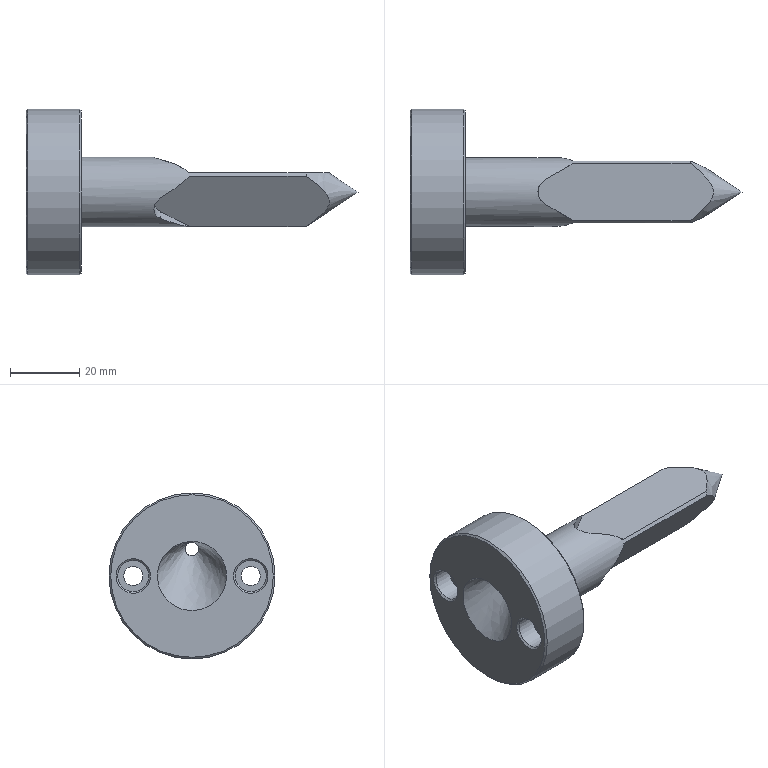NC program | NX | posted with a generic post | part box 96 x 48 x 48 mm
Lines 1 to 853 of 9730:
N10 G17 G21 G94 G90
(ZLEVEL_PROFILE , TOOL : D8)
N12 T08 M6
N14 G54
N16 G17 G0 G90 X5.071 Y-2.683 B0. C0. S3500 M3
N18 G43 Z30. H8
N20 Z1.5
N22 G94 G1 X5.428 Y-2.048 Z1.462 F1000.
N24 X5.805 Y-0.502 Z1.378
N26 X5.75 Y1.087 Z1.295
N28 X5.431 Y2.226 Z1.233
N30 X4.665 Y3.598 Z1.151
N32 X3.56 Y4.716 Z1.068
N34 X2.196 Y5.499 Z0.986
N36 X0.673 Y5.889 Z0.904
N38 X-0.898 Y5.858 Z0.821
N40 X-2.405 Y5.41 Z0.739
N42 X-3.737 Y4.575 Z0.656
N44 X-4.563 Y3.73 Z0.595
N46 X-5.369 Y2.38 Z0.512
N48 X-5.785 Y0.864 Z0.43
N50 X-5.781 Y-0.708 Z0.347
N52 X-5.357 Y-2.222 Z0.265
N54 X-4.545 Y-3.568 Z0.183
N56 X-3.403 Y-4.648 Z0.1
N58 X-2.014 Y-5.384 Z0.018
N60 X-0.869 Y-5.678 Z-0.044
N62 X-0.591 Y-5.713 Z-0.059
N64 X0. Z-0.09
N66 G3 X5.805 Y0.093 R5.805 F2200.
N68 X0. Y-5.713 R-5.805
N70 G1 X0.32 Y-5.694 Z-0.095
N72 X0.639 Y-5.66 Z-0.101
N74 X0.955 Y-5.609 Z-0.107
N76 X1.267 Y-5.538 Z-0.112
N78 X1.575 Y-5.454 Z-0.118
N80 X1.877 Y-5.349 Z-0.123
N82 X2.173 Y-5.232 Z-0.129
N84 X2.46 Y-5.093 Z-0.135
N86 X2.742 Y-4.948 Z-0.14
N88 X3.01 Y-4.777 Z-0.146
N90 X3.276 Y-4.605 Z-0.151
N92 X3.523 Y-4.406 Z-0.157
N94 X3.769 Y-4.207 Z-0.163
N96 X3.991 Y-3.982 Z-0.168
N98 X4.214 Y-3.758 Z-0.174
N100 X4.419 Y-3.517 Z-0.18
N102 G3 X0. Y-5.593 R-5.742
N104 G1 X0.32 Y-5.575 Z-0.185
N106 X0.639 Y-5.54 Z-0.191
N108 X0.955 Y-5.488 Z-0.196
N110 X1.267 Y-5.416 Z-0.202
N112 X1.575 Y-5.332 Z-0.208
N114 X1.876 Y-5.225 Z-0.213
N116 X2.171 Y-5.107 Z-0.219
N118 X2.458 Y-4.967 Z-0.224
N120 X2.739 Y-4.821 Z-0.23
N122 X3.006 Y-4.648 Z-0.236
N124 X3.271 Y-4.475 Z-0.241
N126 X3.516 Y-4.273 Z-0.247
N128 X3.761 Y-4.073 Z-0.252
N130 X3.981 Y-3.845 Z-0.258
N132 X4.203 Y-3.62 Z-0.264
N134 X4.406 Y-3.378 Z-0.269
N136 G3 X0. Y-5.473 R-5.681
N138 G1 X0.32 Y-5.455 Z-0.275
N140 X0.639 Y-5.42 Z-0.281
N142 X0.955 Y-5.366 Z-0.286
N144 X1.267 Y-5.294 Z-0.292
N146 X1.574 Y-5.21 Z-0.297
N148 X1.875 Y-5.101 Z-0.303
N150 X2.169 Y-4.981 Z-0.309
N152 X2.456 Y-4.842 Z-0.314
N154 X2.736 Y-4.692 Z-0.32
N156 X3.002 Y-4.519 Z-0.325
N158 X3.265 Y-4.343 Z-0.331
N160 X3.509 Y-4.14 Z-0.337
N162 X3.752 Y-3.938 Z-0.342
N164 X3.97 Y-3.709 Z-0.348
N166 X4.191 Y-3.483 Z-0.353
N168 X4.39 Y-3.238 Z-0.359
N170 G3 X0. Y-5.352 R-5.619
N172 G1 X0.32 Y-5.334 Z-0.365
N174 X0.639 Y-5.299 Z-0.37
N176 X0.955 Y-5.245 Z-0.376
N178 X1.267 Y-5.172 Z-0.382
N180 X1.574 Y-5.087 Z-0.387
N182 X1.874 Y-4.977 Z-0.393
N184 X2.168 Y-4.855 Z-0.398
N186 X2.454 Y-4.716 Z-0.404
N188 X2.732 Y-4.563 Z-0.41
N190 X2.999 Y-4.389 Z-0.415
N192 X3.26 Y-4.211 Z-0.421
N194 X3.503 Y-4.007 Z-0.426
N196 X3.743 Y-3.802 Z-0.432
N198 X3.96 Y-3.571 Z-0.438
N200 X4.179 Y-3.343 Z-0.443
N202 X4.376 Y-3.097 Z-0.449
N204 G3 X0. Y-5.23 R-5.556
N206 G1 X0.32 Y-5.214 Z-0.454
N208 X0.64 Y-5.179 Z-0.46
N210 X0.955 Y-5.123 Z-0.466
N212 X1.267 Y-5.05 Z-0.471
N214 X1.574 Y-4.963 Z-0.477
N216 X1.874 Y-4.853 Z-0.483
N218 X2.167 Y-4.729 Z-0.488
N220 X2.453 Y-4.591 Z-0.494
N222 X2.729 Y-4.434 Z-0.499
N224 X2.996 Y-4.26 Z-0.505
N226 X3.255 Y-4.078 Z-0.511
N228 X3.497 Y-3.874 Z-0.516
N230 X3.734 Y-3.665 Z-0.522
N232 X3.95 Y-3.433 Z-0.527
N234 X4.166 Y-3.203 Z-0.533
N236 X4.36 Y-2.954 Z-0.539
N238 G3 X0. Y-5.11 R-5.493
N240 G1 X0.32 Y-5.094 Z-0.544
N242 X0.639 Y-5.058 Z-0.55
N244 X0.954 Y-5.001 Z-0.555
N246 X1.266 Y-4.927 Z-0.561
N248 X1.573 Y-4.84 Z-0.567
N250 X1.872 Y-4.728 Z-0.572
N252 X2.165 Y-4.603 Z-0.578
N254 X2.451 Y-4.464 Z-0.584
N256 X2.726 Y-4.305 Z-0.589
N258 X2.992 Y-4.132 Z-0.595
N260 X3.248 Y-3.946 Z-0.6
N262 X3.49 Y-3.74 Z-0.606
N264 X3.725 Y-3.529 Z-0.612
N266 X3.938 Y-3.295 Z-0.617
N268 X4.152 Y-3.063 Z-0.623
N270 X4.344 Y-2.812 Z-0.628
N272 G3 X-0.001 Y-4.989 R-5.43
N274 G1 X0.32 Y-4.974 Z-0.634
N276 X0.64 Y-4.938 Z-0.64
N278 X0.954 Y-4.88 Z-0.645
N280 X1.266 Y-4.805 Z-0.651
N282 X1.572 Y-4.716 Z-0.657
N284 X1.871 Y-4.603 Z-0.662
N286 X2.164 Y-4.478 Z-0.668
N288 X2.449 Y-4.336 Z-0.673
N290 X2.723 Y-4.176 Z-0.679
N292 X2.989 Y-4.002 Z-0.685
N294 X3.243 Y-3.813 Z-0.69
N296 X3.483 Y-3.605 Z-0.696
N298 X3.716 Y-3.392 Z-0.701
N300 X3.928 Y-3.157 Z-0.707
N302 X4.139 Y-2.922 Z-0.713
N304 X4.328 Y-2.669 Z-0.718
N306 G3 X-0.001 Y-4.868 R-5.368
N308 G1 X0.32 Y-4.854 Z-0.724
N310 X0.64 Y-4.817 Z-0.729
N312 X0.954 Y-4.758 Z-0.735
N314 X1.266 Y-4.683 Z-0.741
N316 X1.572 Y-4.593 Z-0.746
N318 X1.87 Y-4.477 Z-0.752
N320 X2.163 Y-4.353 Z-0.758
N322 X2.446 Y-4.208 Z-0.763
N324 X2.721 Y-4.048 Z-0.769
N326 X2.985 Y-3.872 Z-0.774
N328 X3.238 Y-3.681 Z-0.78
N330 X3.476 Y-3.472 Z-0.786
N332 X3.707 Y-3.256 Z-0.791
N334 X3.917 Y-3.019 Z-0.797
N336 X4.126 Y-2.781 Z-0.802
N338 X4.315 Y-2.529 Z-0.808
N340 G3 X-0.001 Y-4.749 R-5.306
N342 G1 X0.32 Y-4.734 Z-0.814
N344 X0.639 Y-4.697 Z-0.819
N346 X0.954 Y-4.637 Z-0.825
N348 X1.265 Y-4.562 Z-0.831
N350 X1.571 Y-4.47 Z-0.836
N352 X1.868 Y-4.352 Z-0.842
N354 X2.16 Y-4.227 Z-0.847
N356 X2.442 Y-4.08 Z-0.853
N358 X2.716 Y-3.919 Z-0.859
N360 X2.979 Y-3.741 Z-0.864
N362 X3.23 Y-3.549 Z-0.87
N364 X3.468 Y-3.339 Z-0.875
N366 X3.696 Y-3.121 Z-0.881
N368 X3.904 Y-2.883 Z-0.887
N370 X4.109 Y-2.643 Z-0.892
N372 X4.297 Y-2.389 Z-0.898
N374 G3 X-0.001 Y-4.632 R-5.246
N376 G1 X0.32 Y-4.614 Z-0.904
N378 X0.639 Y-4.576 Z-0.909
N380 X0.953 Y-4.515 Z-0.915
N382 X1.264 Y-4.44 Z-0.92
N384 X1.569 Y-4.347 Z-0.926
N386 X1.865 Y-4.228 Z-0.932
N388 X2.157 Y-4.102 Z-0.937
N390 X2.438 Y-3.952 Z-0.943
N392 X2.711 Y-3.791 Z-0.948
N394 X2.972 Y-3.61 Z-0.954
N396 X3.223 Y-3.417 Z-0.96
N398 X3.46 Y-3.207 Z-0.965
N400 X3.685 Y-2.986 Z-0.971
N402 X3.891 Y-2.746 Z-0.976
N404 X4.093 Y-2.503 Z-0.982
N406 X4.277 Y-2.247 Z-0.988
N408 G3 X-0.001 Y-4.507 R-5.182
N410 G1 X0.32 Y-4.494 Z-0.993
N412 X0.639 Y-4.455 Z-0.999
N414 X0.954 Y-4.394 Z-1.005
N416 X1.265 Y-4.318 Z-1.01
N418 X1.569 Y-4.223 Z-1.016
N420 X1.865 Y-4.101 Z-1.021
N422 X2.157 Y-3.975 Z-1.027
N424 X2.436 Y-3.822 Z-1.033
N426 X2.709 Y-3.661 Z-1.038
N428 X2.968 Y-3.477 Z-1.044
N430 X3.218 Y-3.283 Z-1.049
N432 X3.453 Y-3.07 Z-1.055
N434 X3.676 Y-2.847 Z-1.061
N436 X3.882 Y-2.607 Z-1.066
N438 X4.078 Y-2.359 Z-1.072
N440 X4.259 Y-2.1 Z-1.078
N442 G3 X-0.001 Y-4.384 R-5.118
N444 G1 X0.32 Y-4.374 Z-1.083
N446 X0.64 Y-4.335 Z-1.089
N448 X0.954 Y-4.272 Z-1.094
N450 X1.265 Y-4.196 Z-1.1
N452 X1.569 Y-4.099 Z-1.106
N454 X1.864 Y-3.975 Z-1.111
N456 X2.156 Y-3.849 Z-1.117
N458 X2.434 Y-3.693 Z-1.122
N460 X2.707 Y-3.531 Z-1.128
N462 X2.964 Y-3.344 Z-1.134
N464 X3.213 Y-3.15 Z-1.139
N466 X3.445 Y-2.933 Z-1.145
N468 X3.666 Y-2.708 Z-1.151
N470 X3.871 Y-2.466 Z-1.156
N472 X4.063 Y-2.216 Z-1.162
N474 X4.24 Y-1.955 Z-1.167
N476 G3 X-0.001 Y-4.266 R-5.058
N478 G1 X0.32 Y-4.253 Z-1.173
N480 X0.639 Y-4.214 Z-1.179
N482 X0.953 Y-4.15 Z-1.184
N484 X1.265 Y-4.074 Z-1.19
N486 X1.567 Y-3.974 Z-1.195
N488 X1.862 Y-3.849 Z-1.201
N490 X2.154 Y-3.723 Z-1.207
N492 X2.43 Y-3.564 Z-1.212
N494 X2.703 Y-3.403 Z-1.218
N496 X2.957 Y-3.213 Z-1.224
N498 X3.206 Y-3.017 Z-1.229
N500 X3.434 Y-2.797 Z-1.235
N502 X3.655 Y-2.571 Z-1.24
N504 X3.855 Y-2.326 Z-1.246
N506 X4.047 Y-2.076 Z-1.252
N508 X4.219 Y-1.811 Z-1.257
N510 G3 X-0.001 Y-4.144 R-4.995
N512 G1 X0.32 Y-4.133 Z-1.263
N514 X0.639 Y-4.093 Z-1.268
N516 X0.953 Y-4.028 Z-1.274
N518 X1.265 Y-3.953 Z-1.28
N520 X1.566 Y-3.848 Z-1.285
N522 X1.861 Y-3.723 Z-1.291
N524 X2.152 Y-3.596 Z-1.297
N526 X2.427 Y-3.436 Z-1.302
N528 X2.699 Y-3.272 Z-1.308
N530 X2.951 Y-3.079 Z-1.313
N532 X3.199 Y-2.882 Z-1.319
N534 X3.424 Y-2.659 Z-1.325
N536 X3.646 Y-2.433 Z-1.33
N538 X3.839 Y-2.183 Z-1.336
N540 X4.032 Y-1.933 Z-1.341
N542 X4.203 Y-1.667 Z-1.347
N544 G3 X-0.001 Y-4.025 R-4.933
N546 G1 X0.32 Y-4.013 Z-1.353
N548 X0.639 Y-3.973 Z-1.358
N550 X0.952 Y-3.906 Z-1.364
N552 X1.264 Y-3.831 Z-1.37
N554 X1.564 Y-3.723 Z-1.375
N556 X1.859 Y-3.599 Z-1.381
N558 X2.148 Y-3.468 Z-1.386
N560 X2.423 Y-3.308 Z-1.392
N562 X2.693 Y-3.141 Z-1.398
N564 X2.943 Y-2.946 Z-1.403
N566 X3.189 Y-2.747 Z-1.409
N568 X3.411 Y-2.522 Z-1.414
N570 X3.632 Y-2.296 Z-1.42
N572 X3.821 Y-2.042 Z-1.426
N574 X4.013 Y-1.792 Z-1.431
N576 X4.184 Y-1.527 Z-1.437
N578 G3 X-0.001 Y-3.907 R-4.875
N580 G1 X0.32 Y-3.893 Z-1.443
N582 X0.639 Y-3.852 Z-1.448
N584 X0.952 Y-3.784 Z-1.454
N586 X1.263 Y-3.709 Z-1.459
N588 X1.562 Y-3.598 Z-1.465
N590 X1.857 Y-3.475 Z-1.471
N592 X2.144 Y-3.34 Z-1.476
N594 X2.418 Y-3.18 Z-1.482
N596 X2.686 Y-3.01 Z-1.487
N598 X2.936 Y-2.814 Z-1.493
N600 X3.178 Y-2.612 Z-1.499
N602 X3.398 Y-2.385 Z-1.504
N604 X3.616 Y-2.158 Z-1.51
N606 X3.802 Y-1.902 Z-1.516
N608 X3.992 Y-1.65 Z-1.521
N610 X4.157 Y-1.382 Z-1.527
N612 G3 X4.478 Y2.777 R4.813
N614 X-4.702 Y2.09 R4.818
N616 X-0.001 Y-3.782 R4.813
N618 G1 X0.32 Y-3.773 Z-1.532
N620 X0.639 Y-3.731 Z-1.538
N622 X0.952 Y-3.661 Z-1.544
N624 X1.264 Y-3.586 Z-1.549
N626 X1.562 Y-3.473 Z-1.555
N628 X1.857 Y-3.35 Z-1.561
N630 X2.143 Y-3.21 Z-1.566
N632 X2.417 Y-3.049 Z-1.572
N634 X2.682 Y-2.875 Z-1.577
N636 X2.931 Y-2.679 Z-1.583
N638 X3.171 Y-2.474 Z-1.589
N640 X3.39 Y-2.245 Z-1.594
N642 X3.605 Y-2.014 Z-1.6
N644 X3.788 Y-1.757 Z-1.605
N646 X3.976 Y-1.503 Z-1.611
N648 X4.139 Y-1.233 Z-1.617
N650 G3 X-0.002 Y-3.665 R-4.747
N652 G1 X0.32 Y-3.653 Z-1.622
N654 X0.639 Y-3.61 Z-1.628
N656 X0.951 Y-3.539 Z-1.634
N658 X1.263 Y-3.464 Z-1.639
N660 X1.56 Y-3.348 Z-1.645
N662 X1.854 Y-3.225 Z-1.65
N664 X2.137 Y-3.082 Z-1.656
N666 X2.411 Y-2.921 Z-1.662
N668 X2.674 Y-2.744 Z-1.667
N670 X2.921 Y-2.546 Z-1.673
N672 X3.16 Y-2.34 Z-1.678
N674 X3.376 Y-2.109 Z-1.684
N676 X3.59 Y-1.877 Z-1.69
N678 X3.769 Y-1.618 Z-1.695
N680 X3.956 Y-1.363 Z-1.701
N682 X4.114 Y-1.09 Z-1.707
N684 G3 X-0.002 Y-3.547 R-4.687
N686 G1 X0.319 Y-3.533 Z-1.712
N688 X0.638 Y-3.489 Z-1.718
N690 X0.95 Y-3.418 Z-1.723
N692 X1.261 Y-3.341 Z-1.729
N694 X1.557 Y-3.222 Z-1.735
N696 X1.851 Y-3.099 Z-1.74
N698 X2.133 Y-2.953 Z-1.746
N700 X2.407 Y-2.793 Z-1.751
N702 X2.667 Y-2.613 Z-1.757
N704 X2.913 Y-2.414 Z-1.763
N706 X3.15 Y-2.205 Z-1.768
N708 X3.364 Y-1.972 Z-1.774
N710 X3.576 Y-1.739 Z-1.78
N712 X3.753 Y-1.478 Z-1.785
N714 X3.934 Y-1.219 Z-1.791
N716 X4.085 Y-0.943 Z-1.796
N718 G3 X-0.002 Y-3.421 R-4.622
N720 G1 X0.32 Y-3.412 Z-1.802
N722 X0.639 Y-3.367 Z-1.808
N724 X0.951 Y-3.296 Z-1.813
N726 X1.262 Y-3.217 Z-1.819
N728 X1.557 Y-3.095 Z-1.825
N730 X1.852 Y-2.973 Z-1.83
N732 X2.132 Y-2.824 Z-1.836
N734 X2.405 Y-2.661 Z-1.841
N736 X2.665 Y-2.48 Z-1.847
N738 X2.909 Y-2.278 Z-1.853
N740 X3.145 Y-2.068 Z-1.858
N742 X3.356 Y-1.832 Z-1.864
N744 X3.566 Y-1.596 Z-1.869
N746 X3.742 Y-1.334 Z-1.875
N748 X3.914 Y-1.069 Z-1.881
N750 X4.066 Y-0.792 Z-1.886
N752 G3 X-0.002 Y-3.301 R-4.561
N754 G1 X0.319 Y-3.292 Z-1.892
N756 X0.638 Y-3.246 Z-1.898
N758 X0.951 Y-3.174 Z-1.903
N760 X1.261 Y-3.093 Z-1.909
N762 X1.555 Y-2.97 Z-1.914
N764 X1.85 Y-2.847 Z-1.92
N766 X2.129 Y-2.697 Z-1.926
N768 X2.401 Y-2.532 Z-1.931
N770 X2.66 Y-2.35 Z-1.937
N772 X2.902 Y-2.146 Z-1.943
N774 X3.137 Y-1.935 Z-1.948
N776 X3.346 Y-1.697 Z-1.954
N778 X3.549 Y-1.456 Z-1.959
N780 X3.724 Y-1.193 Z-1.965
N782 X3.891 Y-0.925 Z-1.971
N784 X4.041 Y-0.648 Z-1.976
N786 G3 X-0.002 Y-3.179 R-4.499
N788 G1 X0.32 Y-3.172 Z-1.982
N790 X0.638 Y-3.124 Z-1.987
N792 X0.951 Y-3.053 Z-1.993
N794 X1.26 Y-2.968 Z-1.999
N796 X1.554 Y-2.844 Z-2.004
N798 X1.848 Y-2.721 Z-2.01
N800 X2.127 Y-2.569 Z-2.016
N802 X2.397 Y-2.403 Z-2.021
N804 X2.656 Y-2.22 Z-2.027
N806 X2.896 Y-2.013 Z-2.032
N808 X3.127 Y-1.798 Z-2.038
N810 X3.337 Y-1.561 Z-2.044
N812 X3.533 Y-1.314 Z-2.049
N814 X3.706 Y-1.05 Z-2.055
N816 X3.869 Y-0.78 Z-2.061
N818 X4.011 Y-0.499 Z-2.066
N820 G3 X-0.002 Y-3.058 R-4.434
N822 G1 X0.319 Y-3.052 Z-2.072
N824 X0.638 Y-3.002 Z-2.077
N826 X0.95 Y-2.932 Z-2.083
N828 X1.259 Y-2.843 Z-2.089
N830 X1.553 Y-2.719 Z-2.094
N832 X1.846 Y-2.595 Z-2.1
N834 X2.125 Y-2.442 Z-2.105
N836 X2.394 Y-2.273 Z-2.111
N838 X2.652 Y-2.09 Z-2.117
N840 X2.89 Y-1.88 Z-2.122
N842 X3.117 Y-1.66 Z-2.128
N844 X3.324 Y-1.421 Z-2.134
N846 X3.518 Y-1.172 Z-2.139
N848 X3.682 Y-0.903 Z-2.145
N850 X3.849 Y-0.634 Z-2.15
N852 X3.987 Y-0.351 Z-2.156
N854 G3 X-0.002 Y-2.942 R-4.376
N856 G1 X0.319 Y-2.932 Z-2.162
N858 X0.637 Y-2.881 Z-2.167
N860 X0.949 Y-2.811 Z-2.173
N862 X1.256 Y-2.718 Z-2.179
N864 X1.55 Y-2.596 Z-2.184
N866 X1.843 Y-2.469 Z-2.19
N868 X2.121 Y-2.317 Z-2.195
N870 X2.387 Y-2.144 Z-2.201
N872 X2.643 Y-1.958 Z-2.207
N874 X2.879 Y-1.747 Z-2.212
N876 X3.104 Y-1.525 Z-2.218
N878 X3.305 Y-1.282 Z-2.223
N880 X3.5 Y-1.034 Z-2.229
N882 X3.657 Y-0.76 Z-2.235
N884 X3.823 Y-0.491 Z-2.24
N886 X3.961 Y-0.208 Z-2.246
N888 G3 X-0.002 Y-2.82 R-4.315
N890 G1 X0.319 Y-2.811 Z-2.252
N892 X0.637 Y-2.759 Z-2.257
N894 X0.949 Y-2.69 Z-2.263
N896 X1.255 Y-2.593 Z-2.268
N898 X1.549 Y-2.472 Z-2.274
N900 X1.84 Y-2.341 Z-2.28
N902 X2.119 Y-2.192 Z-2.285
N904 X2.382 Y-2.013 Z-2.291
N906 X2.636 Y-1.825 Z-2.297
N908 X2.871 Y-1.612 Z-2.302
N910 X3.093 Y-1.389 Z-2.308
N912 X3.288 Y-1.14 Z-2.313
N914 X3.483 Y-0.892 Z-2.319
N916 X3.659 Y-0.63 Z-2.325
N918 X3.798 Y-0.348 Z-2.33
N920 X3.925 Y-0.059 Z-2.336
N922 G3 X-0.003 Y-2.695 R-4.25
N924 G1 X0.319 Y-2.691 Z-2.342
N926 X0.638 Y-2.637 Z-2.347
N928 X0.95 Y-2.569 Z-2.353
N930 X1.255 Y-2.466 Z-2.358
N932 X1.55 Y-2.348 Z-2.364
N934 X1.839 Y-2.211 Z-2.37
N936 X2.119 Y-2.063 Z-2.375
N938 X2.379 Y-1.88 Z-2.381
N940 X2.632 Y-1.69 Z-2.386
N942 X2.862 Y-1.472 Z-2.392
N944 X3.084 Y-1.248 Z-2.398
N946 X3.274 Y-0.994 Z-2.403
N948 X3.468 Y-0.746 Z-2.409
N950 X3.616 Y-0.467 Z-2.415
N952 X3.773 Y-0.193 Z-2.42
N954 X3.892 Y0.099 Z-2.426
N956 G3 X-0.003 Y-2.573 R-4.186
N958 G1 X0.319 Y-2.571 Z-2.431
N960 X0.637 Y-2.515 Z-2.437
N962 X0.951 Y-2.449 Z-2.443
N964 X1.254 Y-2.34 Z-2.448
N966 X1.551 Y-2.224 Z-2.454
N968 X1.837 Y-2.083 Z-2.46
N970 X2.116 Y-1.933 Z-2.465
N972 X2.376 Y-1.749 Z-2.471
N974 X2.626 Y-1.555 Z-2.476
N976 X2.852 Y-1.332 Z-2.482
N978 X3.073 Y-1.106 Z-2.488
N980 X3.26 Y-0.851 Z-2.493
N982 X3.453 Y-0.601 Z-2.499
N984 X3.597 Y-0.32 Z-2.505
N986 X3.744 Y-0.04 Z-2.51
N988 X3.858 Y0.254 Z-2.516
N990 G3 X-0.003 Y-2.45 R-4.12
N992 G1 X0.32 Y-2.451 Z-2.521
N994 X0.637 Y-2.393 Z-2.527
N996 X0.951 Y-2.328 Z-2.533
N998 X1.253 Y-2.214 Z-2.538
N1000 X1.551 Y-2.102 Z-2.544
N1002 X1.835 Y-1.955 Z-2.549
N1004 X2.114 Y-1.803 Z-2.555
N1006 X2.372 Y-1.617 Z-2.561
N1008 X2.618 Y-1.418 Z-2.566
N1010 X2.842 Y-1.193 Z-2.572
N1012 X3.062 Y-0.966 Z-2.578
N1014 X3.247 Y-0.709 Z-2.583
N1016 X3.433 Y-0.454 Z-2.589
N1018 X3.573 Y-0.171 Z-2.594
N1020 X3.717 Y0.111 Z-2.6
N1022 X3.838 Y0.403 Z-2.606
N1024 G3 X-0.003 Y-2.339 R-4.066
N1026 G1 X0.318 Y-2.33 Z-2.611
N1028 X0.636 Y-2.271 Z-2.617
N1030 X0.949 Y-2.208 Z-2.623
N1032 X1.248 Y-2.09 Z-2.628
N1034 X1.547 Y-1.981 Z-2.634
N1036 X1.828 Y-1.831 Z-2.639
N1038 X2.104 Y-1.675 Z-2.645
N1040 X2.36 Y-1.488 Z-2.651
N1042 X2.604 Y-1.288 Z-2.656
N1044 X2.825 Y-1.062 Z-2.662
N1046 X3.045 Y-0.836 Z-2.668
N1048 X3.227 Y-0.578 Z-2.673
N1050 X3.404 Y-0.319 Z-2.679
N1052 X3.541 Y-0.035 Z-2.684
N1054 X3.684 Y0.246 Z-2.69
N1056 X3.799 Y0.539 Z-2.696
N1058 G3 X-0.003 Y-2.215 R-4.003
N1060 G1 X0.319 Y-2.21 Z-2.701
N1062 X0.636 Y-2.148 Z-2.707
N1064 X0.949 Y-2.086 Z-2.713
N1066 X1.248 Y-1.964 Z-2.718
N1068 X1.546 Y-1.854 Z-2.724
N1070 X1.827 Y-1.704 Z-2.729
N1072 X2.1 Y-1.543 Z-2.735
N1074 X2.354 Y-1.353 Z-2.741
N1076 X2.597 Y-1.152 Z-2.746
N1078 X2.817 Y-0.924 Z-2.752
N1080 X3.034 Y-0.696 Z-2.758
N1082 X3.213 Y-0.436 Z-2.763
N1084 X3.384 Y-0.173 Z-2.769
N1086 X3.517 Y0.113 Z-2.774
N1088 X3.66 Y0.395 Z-2.78
N1090 X3.754 Y0.695 Z-2.786
N1092 G3 X-0.003 Y-2.087 R-3.934
N1094 G1 X0.159 Y-2.098 Z-2.788
N1096 X0.319 Y-2.09 Z-2.791
N1098 X0.478 Y-2.063 Z-2.794
N1100 X0.637 Y-2.026 Z-2.797
N1102 X0.794 Y-1.994 Z-2.8
N1104 X0.951 Y-1.963 Z-2.802
N1106 X1.1 Y-1.9 Z-2.805
N1108 X1.249 Y-1.839 Z-2.808
N1110 X1.547 Y-1.727 Z-2.814
N1112 X1.829 Y-1.577 Z-2.819
N1114 X2.098 Y-1.409 Z-2.825
N1116 X2.351 Y-1.217 Z-2.831
N1118 X2.595 Y-1.015 Z-2.836
N1120 X2.812 Y-0.785 Z-2.842
N1122 X3.022 Y-0.549 Z-2.847
N1124 X3.198 Y-0.286 Z-2.853
N1126 X3.37 Y-0.021 Z-2.859
N1128 X3.522 Y0.256 Z-2.864
N1130 X3.629 Y0.553 Z-2.87
N1132 X3.714 Y0.858 Z-2.876
N1134 G3 X-0.004 Y-1.959 R-3.87
N1136 G1 X0.16 Y-1.978 Z-2.878
N1138 X0.32 Y-1.969 Z-2.881
N1140 X0.479 Y-1.94 Z-2.884
N1142 X0.638 Y-1.904 Z-2.887
N1144 X0.951 Y-1.837 Z-2.892
N1146 X1.251 Y-1.714 Z-2.898
N1148 X1.547 Y-1.597 Z-2.904
N1150 X1.83 Y-1.448 Z-2.909
N1152 X2.097 Y-1.276 Z-2.915
N1154 X2.349 Y-1.081 Z-2.921
N1156 X2.594 Y-0.879 Z-2.926
N1158 X2.809 Y-0.646 Z-2.932
N1160 X3.011 Y-0.403 Z-2.937
N1162 X3.182 Y-0.135 Z-2.943
N1164 X3.272 Y-0.005 Z-2.946
N1166 X3.354 Y0.13 Z-2.949
N1168 X3.421 Y0.272 Z-2.951
N1170 X3.471 Y0.424 Z-2.954
N1172 X3.595 Y0.715 Z-2.96
N1174 X3.677 Y1.02 Z-2.966
N1176 G3 X2.853 Y4.496 R3.83
N1178 X-2.028 Y-1.292 R-3.824
N1180 X-0.004 Y-1.854 R3.83
N1182 G1 X0.157 Y-1.858 Z-2.968
N1184 X0.318 Y-1.849 Z-2.971
N1186 X0.476 Y-1.819 Z-2.974
N1188 X0.635 Y-1.783 Z-2.977
N1190 X0.946 Y-1.713 Z-2.982
N1192 X1.245 Y-1.592 Z-2.988
N1194 X1.54 Y-1.471 Z-2.994
N1196 X1.821 Y-1.321 Z-2.999
N1198 X2.088 Y-1.15 Z-3.005
N1200 X2.338 Y-0.954 Z-3.011
N1202 X2.579 Y-0.748 Z-3.016
N1204 X2.794 Y-0.515 Z-3.022
N1206 X2.993 Y-0.269 Z-3.027
N1208 X3.156 Y0.003 Z-3.033
N1210 X3.249 Y0.132 Z-3.036
N1212 X3.328 Y0.269 Z-3.039
N1214 X3.39 Y0.414 Z-3.041
N1216 X3.434 Y0.568 Z-3.044
N1218 X3.557 Y0.86 Z-3.05
N1220 X3.649 Y1.162 Z-3.056
N1222 G3 X-0.004 Y-1.733 R-3.756
N1224 G1 X0.157 Y-1.738 Z-3.058
N1226 X0.318 Y-1.729 Z-3.061
N1228 X0.476 Y-1.697 Z-3.064
N1230 X0.634 Y-1.662 Z-3.067
N1232 X0.944 Y-1.587 Z-3.072
N1234 X1.243 Y-1.469 Z-3.078
N1236 X1.535 Y-1.345 Z-3.084
N1238 X1.815 Y-1.193 Z-3.089
N1240 X2.082 Y-1.023 Z-3.095
N1242 X2.329 Y-0.825 Z-3.101
N1244 X2.565 Y-0.615 Z-3.106
N1246 X2.774 Y-0.378 Z-3.112
N1248 X2.974 Y-0.135 Z-3.117
N1250 X3.131 Y0.139 Z-3.123
N1252 X3.295 Y0.409 Z-3.129
N1254 X3.422 Y0.697 Z-3.134
N1256 X3.519 Y0.996 Z-3.14
N1258 X3.595 Y1.302 Z-3.146
N1260 G3 X-0.005 Y-1.607 R-3.69
N1262 G1 X0.158 Y-1.617 Z-3.148
N1264 X0.318 Y-1.608 Z-3.151
N1266 X0.476 Y-1.575 Z-3.154
N1268 X0.635 Y-1.541 Z-3.157
N1270 X0.944 Y-1.461 Z-3.162
N1272 X1.244 Y-1.346 Z-3.168
N1274 X1.535 Y-1.217 Z-3.174
N1276 X1.814 Y-1.063 Z-3.179
N1278 X2.082 Y-0.893 Z-3.185
N1280 X2.328 Y-0.692 Z-3.191
N1282 X2.558 Y-0.476 Z-3.196
N1284 X2.761 Y-0.232 Z-3.202
N1286 X2.962 Y0.011 Z-3.207
N1288 X3.116 Y0.288 Z-3.213
N1290 X3.27 Y0.564 Z-3.219
N1292 X3.398 Y0.852 Z-3.224
N1294 X3.491 Y1.154 Z-3.23
N1296 X3.559 Y1.464 Z-3.236
N1298 X3.573 Y1.544
N1300 G3 X-0.005 Y-1.489 R-3.631
N1302 G1 X0.157 Y-1.497 Z-3.238
N1304 X0.318 Y-1.488 Z-3.241
N1306 X0.476 Y-1.453 Z-3.244
N1308 X0.634 Y-1.42 Z-3.247
N1310 X0.942 Y-1.335 Z-3.252
N1312 X1.243 Y-1.224 Z-3.258
N1314 X1.532 Y-1.091 Z-3.264
N1316 X1.81 Y-0.936 Z-3.269
N1318 X2.136 Y-0.726 Z-3.276
N1320 X2.319 Y-0.56 Z-3.281
N1322 X2.548 Y-0.343 Z-3.286
N1324 X2.745 Y-0.094 Z-3.292
N1326 X2.853 Y0.022 Z-3.295
N1328 X2.945 Y0.149 Z-3.297
N1330 X3.025 Y0.285 Z-3.3
N1332 X3.09 Y0.431 Z-3.303
N1334 X3.242 Y0.708 Z-3.309
N1336 X3.37 Y0.995 Z-3.314
N1338 X3.446 Y1.302 Z-3.32
N1340 X3.509 Y1.611 Z-3.326
N1342 G3 X-0.005 Y-1.366 R-3.566
N1344 G1 X0.158 Y-1.377 Z-3.328
N1346 X0.318 Y-1.367 Z-3.331
N1348 X0.476 Y-1.331 Z-3.334
N1350 X0.635 Y-1.299 Z-3.337
N1352 X0.942 Y-1.21 Z-3.342
N1354 X1.244 Y-1.101 Z-3.348
N1356 X1.531 Y-0.965 Z-3.354
N1358 X1.808 Y-0.808 Z-3.359
N1360 X2.115 Y-0.602 Z-3.366
N1362 X2.312 Y-0.424 Z-3.371
N1364 X2.538 Y-0.204 Z-3.376
N1366 X2.732 Y0.046 Z-3.382
N1368 X2.839 Y0.164 Z-3.385
N1370 X2.925 Y0.296 Z-3.387
N1372 X3.007 Y0.43 Z-3.39
N1374 X3.066 Y0.579 Z-3.393
N1376 X3.219 Y0.856 Z-3.399
N1378 X3.332 Y1.15 Z-3.404
N1380 X3.403 Y1.458 Z-3.41
N1382 X3.47 Y1.767 Z-3.416
N1384 G3 X-0.005 Y-1.263 R-3.514
N1386 G1 X0.372 Y-1.232 Z-3.422
N1388 X0.631 Y-1.178 Z-3.427
N1390 X0.936 Y-1.086 Z-3.432
N1392 X1.237 Y-0.98 Z-3.438
N1394 X1.556 Y-0.827 Z-3.444
N1396 X1.797 Y-0.685 Z-3.449
N1398 X2.057 Y-0.506 Z-3.455
N1400 X2.292 Y-0.295 Z-3.461
N1402 X2.519 Y-0.076 Z-3.466
N1404 X2.71 Y0.174 Z-3.472
N1406 X2.896 Y0.427 Z-3.477
N1408 X3.034 Y0.71 Z-3.483
N1410 X3.187 Y0.987 Z-3.489
N1412 X3.288 Y1.284 Z-3.494
N1414 X3.357 Y1.592 Z-3.5
N1416 X3.416 Y1.902 Z-3.506
N1418 G3 X-0.005 Y-1.135 R-3.449
N1420 G1 X0.399 Y-1.104 Z-3.513
N1422 X0.632 Y-1.058 Z-3.517
N1424 X0.937 Y-0.961 Z-3.522
N1426 X1.237 Y-0.853 Z-3.528
N1428 X1.563 Y-0.699 Z-3.534
N1430 X1.796 Y-0.554 Z-3.539
N1432 X2.054 Y-0.372 Z-3.545
N1434 X2.285 Y-0.155 Z-3.551
N1436 X2.512 Y0.063 Z-3.556
N1438 X2.7 Y0.317 Z-3.562
N1440 X2.881 Y0.576 Z-3.567
N1442 X3.042 Y0.846 Z-3.573
N1444 X3.15 Y1.118 Z-3.578
N1446 X3.254 Y1.441 Z-3.584
N1448 X3.318 Y1.75 Z-3.59
N1450 X3.361 Y2.062 Z-3.596
N1452 G3 X-0.005 Y-1.011 R-3.382
N1454 G1 X0.416 Y-0.978 Z-3.603
N1456 X0.633 Y-0.937 Z-3.607
N1458 X0.937 Y-0.837 Z-3.612
N1460 X1.237 Y-0.728 Z-3.618
N1462 X1.569 Y-0.572 Z-3.625
N1464 X1.795 Y-0.425 Z-3.629
N1466 X2.049 Y-0.237 Z-3.635
N1468 X2.278 Y-0.018 Z-3.641
N1470 X2.502 Y0.203 Z-3.646
N1472 X2.683 Y0.462 Z-3.652
N1474 X2.779 Y0.588 Z-3.655
N1476 X2.864 Y0.72 Z-3.657
N1478 X2.939 Y0.858 Z-3.66
N1480 X2.99 Y1.009 Z-3.663
N1482 X3.12 Y1.297 Z-3.669
N1484 X3.221 Y1.595 Z-3.674
N1486 X3.27 Y1.907 Z-3.68
N1488 X3.306 Y2.221 Z-3.686
N1490 G3 X-0.005 Y-0.879 R-3.315
N1492 G1 X0.453 Y-0.849 Z-3.694
N1494 X0.636 Y-0.816 Z-3.697
N1496 X0.935 Y-0.714 Z-3.702
N1498 X1.24 Y-0.601 Z-3.708
N1500 X1.574 Y-0.441 Z-3.715
N1502 X1.796 Y-0.294 Z-3.719
N1504 X2.047 Y-0.1 Z-3.725
N1506 X2.275 Y0.121 Z-3.731
N1508 X2.493 Y0.349 Z-3.736
N1510 X2.67 Y0.611 Z-3.742
N1512 X2.851 Y0.871 Z-3.747
N1514 X2.986 Y1.156 Z-3.753
N1516 X3.119 Y1.523 Z-3.76
N1518 X3.183 Y1.756 Z-3.764
N1520 X3.222 Y2.07 Z-3.77
N1522 X3.251 Y2.385 Z-3.776
N1524 G3 X0.721 Y5.666 R3.248
N1526 X-0.005 Y-0.769 R-3.259
N1528 G1 X0.43 Y-0.732 Z-3.783
N1530 X0.634 Y-0.696 Z-3.787
N1532 X0.932 Y-0.592 Z-3.792
N1534 X1.235 Y-0.478 Z-3.798
N1536 X1.549 Y-0.324 Z-3.804
N1538 X1.786 Y-0.163 Z-3.809
N1540 X2.038 Y0.029 Z-3.815
N1542 X2.264 Y0.251 Z-3.821
N1544 X2.477 Y0.484 Z-3.826
N1546 X2.65 Y0.748 Z-3.832
N1548 X2.822 Y1.014 Z-3.838
N1550 X2.957 Y1.299 Z-3.843
N1552 X3.068 Y1.621 Z-3.849
N1554 X3.135 Y1.905 Z-3.854
N1556 X3.171 Y2.219 Z-3.86
N1558 X3.201 Y2.534 Z-3.866
N1560 G3 X-0.005 Y-0.662 R-3.203
N1562 G1 X0.392 Y-0.618 Z-3.873
N1564 X0.631 Y-0.576 Z-3.877
N1566 X0.925 Y-0.471 Z-3.882
N1568 X1.228 Y-0.355 Z-3.888
N1570 X1.53 Y-0.204 Z-3.894
N1572 X1.773 Y-0.036 Z-3.899
N1574 X2.101 Y0.216 Z-3.907
N1576 X2.247 Y0.376 Z-3.911
N1578 X2.455 Y0.611 Z-3.916
N1580 X2.622 Y0.877 Z-3.922
N1582 X2.788 Y1.145 Z-3.928
N1584 X2.923 Y1.428 Z-3.933
N1586 X3.022 Y1.736 Z-3.939
N1588 X3.087 Y2.035 Z-3.944
N1590 X3.111 Y2.349 Z-3.95
N1592 X3.133 Y2.663 Z-3.956
N1594 G3 X-0.005 Y-0.532 R-3.137
N1596 G1 X0.421 Y-0.492 Z-3.963
N1598 X0.633 Y-0.455 Z-3.967
N1600 X0.923 Y-0.349 Z-3.972
N1602 X1.23 Y-0.228 Z-3.978
N1604 X1.534 Y-0.07 Z-3.984
N1606 X1.772 Y0.098 Z-3.989
N1608 X2.09 Y0.343 Z-3.997
N1610 X2.238 Y0.521 Z-4.001
N1612 X2.347 Y0.635 Z-4.004
N1614 X2.448 Y0.755 Z-4.006
N1616 X2.537 Y0.885 Z-4.009
N1618 X2.606 Y1.028 Z-4.012
N1620 X2.768 Y1.3 Z-4.018
N1622 X2.899 Y1.585 Z-4.023
N1624 X2.996 Y1.906 Z-4.029
N1626 X3.05 Y2.199 Z-4.034
N1628 X3.057 Y2.515 Z-4.04
N1630 X3.066 Y2.831 Z-4.046
N1632 G3 X1.408 Y5.38 R3.018
N1634 X-0.006 Y-0.398 R-3.067
N1636 G1 X0.456 Y-0.365 Z-4.054
N1638 X0.634 Y-0.329 Z-4.057
N1640 X0.954 Y-0.218 Z-4.063
N1642 X1.234 Y-0.1 Z-4.068
N1644 X1.549 Y0.07 Z-4.075
N1646 X1.776 Y0.235 Z-4.08
N1648 X2.087 Y0.489 Z-4.087
N1650 X2.238 Y0.67 Z-4.091
N1652 X2.347 Y0.786 Z-4.094
N1654 X2.445 Y0.91 Z-4.096
N1656 X2.53 Y1.044 Z-4.099
N1658 X2.595 Y1.192 Z-4.102
N1660 X2.756 Y1.466 Z-4.108
N1662 X2.87 Y1.76 Z-4.113
N1664 X2.961 Y2.121 Z-4.12
N1666 X3. Y2.379 Z-4.125
N1668 X3.001 Y2.695 Z-4.13
N1670 X2.988 Y3.01 Z-4.136
N1672 G3 X-0.006 Y-0.284 R-3.012
N1674 G1 X0.425 Y-0.249 Z-4.143
N1676 X0.632 Y-0.207 Z-4.147
N1678 X0.965 Y-0.094 Z-4.153
N1680 X1.229 Y0.022 Z-4.158
N1682 X1.551 Y0.201 Z-4.165
N1684 X1.766 Y0.361 Z-4.17
N1686 X2.01 Y0.563 Z-4.175
N1688 X2.218 Y0.802 Z-4.181
N1690 X2.505 Y1.166 Z-4.189
N1692 X2.59 Y1.312 Z-4.192
N1694 X2.75 Y1.654 Z-4.199
N1696 X2.831 Y1.897 Z-4.203
N1698 X2.92 Y2.283 Z-4.21
N1700 X2.947 Y2.52 Z-4.215
N1702 X2.936 Y2.836 Z-4.22
N1704 X2.921 Y3.153 Z-4.226